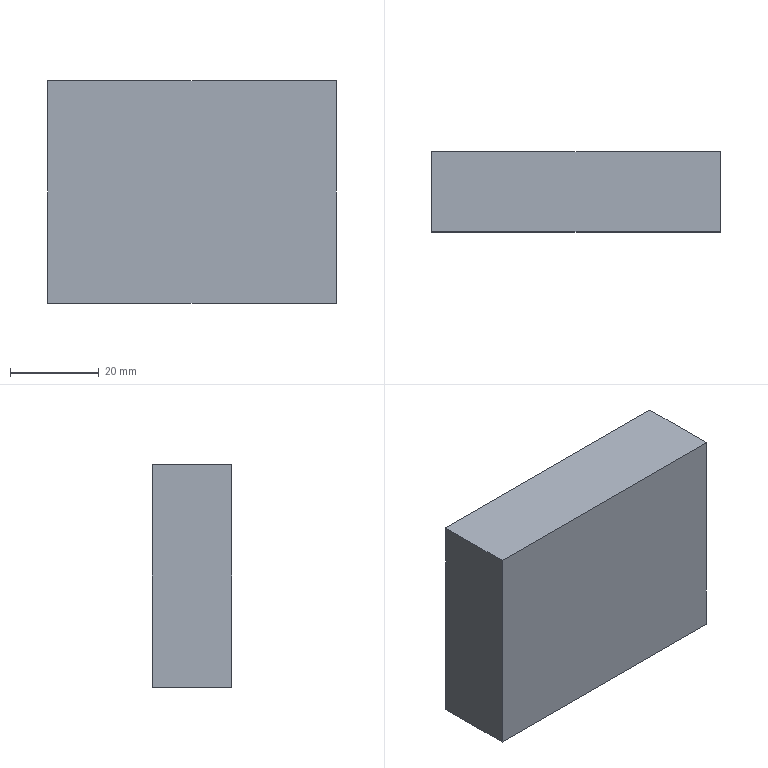Part | STEP file | Superstructure_3_1 | 1 solid | 6 faces | box 65 x 18 x 50 mm | volume 58500 mm3 | plane 6
STEP:
#1=CARTESIAN_POINT('',(0.,0.,0.));
#2=DIRECTION('',(0.,0.,1.));
#3=DIRECTION('',(1.,0.,0.));
#4=AXIS2_PLACEMENT_3D('',#1,#2,#3);
#5=CARTESIAN_POINT('',(-32.5,9.,50.));
#6=VERTEX_POINT('',#5);
#7=CARTESIAN_POINT('',(-32.5,-9.,50.));
#8=VERTEX_POINT('',#7);
#9=CARTESIAN_POINT('',(-32.5,9.,50.));
#10=DIRECTION('',(0.,-1.,0.));
#11=VECTOR('',#10,1.);
#12=LINE('',#9,#11);
#13=CARTESIAN_POINT('',(-32.5,9.,50.));
#14=DIRECTION('',(1.,0.,0.));
#15=DIRECTION('',(0.,0.,-1.));
#16=AXIS2_PLACEMENT_3D('',#13,#14,#15);
#17=PLANE('',#16);
#18=CARTESIAN_POINT('',(0.,0.));
#19=DIRECTION('',(0.,-1.));
#20=VECTOR('',#19,1.);
#21=LINE('',#18,#20);
#22=(GEOMETRIC_REPRESENTATION_CONTEXT(2)PARAMETRIC_REPRESENTATION_CONTEXT()REPRESENTATION_CONTEXT('',''));
#23=DEFINITIONAL_REPRESENTATION('',(#21),#22);
#24=PCURVE('',#17,#23);
#25=CARTESIAN_POINT('',(32.5,9.,50.));
#26=DIRECTION('',(0.,0.,-1.));
#27=DIRECTION('',(-1.,0.,0.));
#28=AXIS2_PLACEMENT_3D('',#25,#26,#27);
#29=PLANE('',#28);
#30=CARTESIAN_POINT('',(65.,0.));
#31=DIRECTION('',(0.,-1.));
#32=VECTOR('',#31,1.);
#33=LINE('',#30,#32);
#34=(GEOMETRIC_REPRESENTATION_CONTEXT(2)PARAMETRIC_REPRESENTATION_CONTEXT()REPRESENTATION_CONTEXT('',''));
#35=DEFINITIONAL_REPRESENTATION('',(#33),#34);
#36=PCURVE('',#29,#35);
#37=SURFACE_CURVE('',#12,(#24,#36),.PCURVE_S1.);
#38=EDGE_CURVE('',#6,#8,#37,.T.);
#39=ORIENTED_EDGE('',*,*,#38,.T.);
#40=CARTESIAN_POINT('',(-32.5,-9.,0.));
#41=VERTEX_POINT('',#40);
#42=CARTESIAN_POINT('',(-32.5,-9.,50.));
#43=DIRECTION('',(0.,0.,-1.));
#44=VECTOR('',#43,1.);
#45=LINE('',#42,#44);
#46=CARTESIAN_POINT('',(0.,-18.));
#47=DIRECTION('',(1.,0.));
#48=VECTOR('',#47,1.);
#49=LINE('',#46,#48);
#50=(GEOMETRIC_REPRESENTATION_CONTEXT(2)PARAMETRIC_REPRESENTATION_CONTEXT()REPRESENTATION_CONTEXT('',''));
#51=DEFINITIONAL_REPRESENTATION('',(#49),#50);
#52=PCURVE('',#17,#51);
#53=CARTESIAN_POINT('',(0.,-9.,25.));
#54=DIRECTION('',(0.,1.,0.));
#55=DIRECTION('',(0.,0.,1.));
#56=AXIS2_PLACEMENT_3D('',#53,#54,#55);
#57=PLANE('',#56);
#58=CARTESIAN_POINT('',(25.,-32.5));
#59=DIRECTION('',(-1.,0.));
#60=VECTOR('',#59,1.);
#61=LINE('',#58,#60);
#62=(GEOMETRIC_REPRESENTATION_CONTEXT(2)PARAMETRIC_REPRESENTATION_CONTEXT()REPRESENTATION_CONTEXT('',''));
#63=DEFINITIONAL_REPRESENTATION('',(#61),#62);
#64=PCURVE('',#57,#63);
#65=SURFACE_CURVE('',#45,(#52,#64),.PCURVE_S1.);
#66=EDGE_CURVE('',#8,#41,#65,.T.);
#67=ORIENTED_EDGE('',*,*,#66,.T.);
#68=CARTESIAN_POINT('',(-32.5,9.,0.));
#69=VERTEX_POINT('',#68);
#70=CARTESIAN_POINT('',(-32.5,9.,0.));
#71=DIRECTION('',(0.,-1.,0.));
#72=VECTOR('',#71,1.);
#73=LINE('',#70,#72);
#74=CARTESIAN_POINT('',(50.,0.));
#75=DIRECTION('',(0.,-1.));
#76=VECTOR('',#75,1.);
#77=LINE('',#74,#76);
#78=(GEOMETRIC_REPRESENTATION_CONTEXT(2)PARAMETRIC_REPRESENTATION_CONTEXT()REPRESENTATION_CONTEXT('',''));
#79=DEFINITIONAL_REPRESENTATION('',(#77),#78);
#80=PCURVE('',#17,#79);
#81=CARTESIAN_POINT('',(-32.5,9.,0.));
#82=DIRECTION('',(0.,0.,1.));
#83=DIRECTION('',(1.,0.,0.));
#84=AXIS2_PLACEMENT_3D('',#81,#82,#83);
#85=PLANE('',#84);
#86=CARTESIAN_POINT('',(0.,0.));
#87=DIRECTION('',(0.,-1.));
#88=VECTOR('',#87,1.);
#89=LINE('',#86,#88);
#90=(GEOMETRIC_REPRESENTATION_CONTEXT(2)PARAMETRIC_REPRESENTATION_CONTEXT()REPRESENTATION_CONTEXT('',''));
#91=DEFINITIONAL_REPRESENTATION('',(#89),#90);
#92=PCURVE('',#85,#91);
#93=SURFACE_CURVE('',#73,(#80,#92),.PCURVE_S1.);
#94=EDGE_CURVE('',#69,#41,#93,.T.);
#95=ORIENTED_EDGE('',*,*,#94,.F.);
#96=CARTESIAN_POINT('',(-32.5,9.,50.));
#97=DIRECTION('',(0.,0.,-1.));
#98=VECTOR('',#97,1.);
#99=LINE('',#96,#98);
#100=CARTESIAN_POINT('',(0.,0.));
#101=DIRECTION('',(1.,0.));
#102=VECTOR('',#101,1.);
#103=LINE('',#100,#102);
#104=(GEOMETRIC_REPRESENTATION_CONTEXT(2)PARAMETRIC_REPRESENTATION_CONTEXT()REPRESENTATION_CONTEXT('',''));
#105=DEFINITIONAL_REPRESENTATION('',(#103),#104);
#106=PCURVE('',#17,#105);
#107=CARTESIAN_POINT('',(0.,9.,25.));
#108=DIRECTION('',(0.,1.,0.));
#109=DIRECTION('',(0.,0.,1.));
#110=AXIS2_PLACEMENT_3D('',#107,#108,#109);
#111=PLANE('',#110);
#112=CARTESIAN_POINT('',(25.,-32.5));
#113=DIRECTION('',(-1.,0.));
#114=VECTOR('',#113,1.);
#115=LINE('',#112,#114);
#116=(GEOMETRIC_REPRESENTATION_CONTEXT(2)PARAMETRIC_REPRESENTATION_CONTEXT()REPRESENTATION_CONTEXT('',''));
#117=DEFINITIONAL_REPRESENTATION('',(#115),#116);
#118=PCURVE('',#111,#117);
#119=SURFACE_CURVE('',#99,(#106,#118),.PCURVE_S1.);
#120=EDGE_CURVE('',#6,#69,#119,.T.);
#121=ORIENTED_EDGE('',*,*,#120,.F.);
#122=EDGE_LOOP('',(#39,#67,#95,#121));
#123=FACE_BOUND('',#122,.F.);
#124=ADVANCED_FACE('',(#123),#17,.F.);
#125=ORIENTED_EDGE('',*,*,#94,.T.);
#126=CARTESIAN_POINT('',(32.5,-9.,0.));
#127=VERTEX_POINT('',#126);
#128=CARTESIAN_POINT('',(-32.5,-9.,0.));
#129=DIRECTION('',(1.,0.,0.));
#130=VECTOR('',#129,1.);
#131=LINE('',#128,#130);
#132=CARTESIAN_POINT('',(0.,-18.));
#133=DIRECTION('',(1.,0.));
#134=VECTOR('',#133,1.);
#135=LINE('',#132,#134);
#136=(GEOMETRIC_REPRESENTATION_CONTEXT(2)PARAMETRIC_REPRESENTATION_CONTEXT()REPRESENTATION_CONTEXT('',''));
#137=DEFINITIONAL_REPRESENTATION('',(#135),#136);
#138=PCURVE('',#85,#137);
#139=CARTESIAN_POINT('',(-25.,-32.5));
#140=DIRECTION('',(0.,1.));
#141=VECTOR('',#140,1.);
#142=LINE('',#139,#141);
#143=(GEOMETRIC_REPRESENTATION_CONTEXT(2)PARAMETRIC_REPRESENTATION_CONTEXT()REPRESENTATION_CONTEXT('',''));
#144=DEFINITIONAL_REPRESENTATION('',(#142),#143);
#145=PCURVE('',#57,#144);
#146=SURFACE_CURVE('',#131,(#138,#145),.PCURVE_S1.);
#147=EDGE_CURVE('',#41,#127,#146,.T.);
#148=ORIENTED_EDGE('',*,*,#147,.T.);
#149=CARTESIAN_POINT('',(32.5,9.,0.));
#150=VERTEX_POINT('',#149);
#151=CARTESIAN_POINT('',(32.5,9.,0.));
#152=DIRECTION('',(0.,-1.,0.));
#153=VECTOR('',#152,1.);
#154=LINE('',#151,#153);
#155=CARTESIAN_POINT('',(65.,0.));
#156=DIRECTION('',(0.,-1.));
#157=VECTOR('',#156,1.);
#158=LINE('',#155,#157);
#159=(GEOMETRIC_REPRESENTATION_CONTEXT(2)PARAMETRIC_REPRESENTATION_CONTEXT()REPRESENTATION_CONTEXT('',''));
#160=DEFINITIONAL_REPRESENTATION('',(#158),#159);
#161=PCURVE('',#85,#160);
#162=CARTESIAN_POINT('',(32.5,9.,0.));
#163=DIRECTION('',(-1.,0.,0.));
#164=DIRECTION('',(0.,0.,1.));
#165=AXIS2_PLACEMENT_3D('',#162,#163,#164);
#166=PLANE('',#165);
#167=CARTESIAN_POINT('',(0.,0.));
#168=DIRECTION('',(0.,-1.));
#169=VECTOR('',#168,1.);
#170=LINE('',#167,#169);
#171=(GEOMETRIC_REPRESENTATION_CONTEXT(2)PARAMETRIC_REPRESENTATION_CONTEXT()REPRESENTATION_CONTEXT('',''));
#172=DEFINITIONAL_REPRESENTATION('',(#170),#171);
#173=PCURVE('',#166,#172);
#174=SURFACE_CURVE('',#154,(#161,#173),.PCURVE_S1.);
#175=EDGE_CURVE('',#150,#127,#174,.T.);
#176=ORIENTED_EDGE('',*,*,#175,.F.);
#177=CARTESIAN_POINT('',(-32.5,9.,0.));
#178=DIRECTION('',(1.,0.,0.));
#179=VECTOR('',#178,1.);
#180=LINE('',#177,#179);
#181=CARTESIAN_POINT('',(0.,0.));
#182=DIRECTION('',(1.,0.));
#183=VECTOR('',#182,1.);
#184=LINE('',#181,#183);
#185=(GEOMETRIC_REPRESENTATION_CONTEXT(2)PARAMETRIC_REPRESENTATION_CONTEXT()REPRESENTATION_CONTEXT('',''));
#186=DEFINITIONAL_REPRESENTATION('',(#184),#185);
#187=PCURVE('',#85,#186);
#188=CARTESIAN_POINT('',(-25.,-32.5));
#189=DIRECTION('',(0.,1.));
#190=VECTOR('',#189,1.);
#191=LINE('',#188,#190);
#192=(GEOMETRIC_REPRESENTATION_CONTEXT(2)PARAMETRIC_REPRESENTATION_CONTEXT()REPRESENTATION_CONTEXT('',''));
#193=DEFINITIONAL_REPRESENTATION('',(#191),#192);
#194=PCURVE('',#111,#193);
#195=SURFACE_CURVE('',#180,(#187,#194),.PCURVE_S1.);
#196=EDGE_CURVE('',#69,#150,#195,.T.);
#197=ORIENTED_EDGE('',*,*,#196,.F.);
#198=EDGE_LOOP('',(#125,#148,#176,#197));
#199=FACE_BOUND('',#198,.F.);
#200=ADVANCED_FACE('',(#199),#85,.F.);
#201=ORIENTED_EDGE('',*,*,#175,.T.);
#202=CARTESIAN_POINT('',(32.5,-9.,50.));
#203=VERTEX_POINT('',#202);
#204=CARTESIAN_POINT('',(32.5,-9.,0.));
#205=DIRECTION('',(0.,0.,1.));
#206=VECTOR('',#205,1.);
#207=LINE('',#204,#206);
#208=CARTESIAN_POINT('',(0.,-18.));
#209=DIRECTION('',(1.,0.));
#210=VECTOR('',#209,1.);
#211=LINE('',#208,#210);
#212=(GEOMETRIC_REPRESENTATION_CONTEXT(2)PARAMETRIC_REPRESENTATION_CONTEXT()REPRESENTATION_CONTEXT('',''));
#213=DEFINITIONAL_REPRESENTATION('',(#211),#212);
#214=PCURVE('',#166,#213);
#215=CARTESIAN_POINT('',(-25.,32.5));
#216=DIRECTION('',(1.,0.));
#217=VECTOR('',#216,1.);
#218=LINE('',#215,#217);
#219=(GEOMETRIC_REPRESENTATION_CONTEXT(2)PARAMETRIC_REPRESENTATION_CONTEXT()REPRESENTATION_CONTEXT('',''));
#220=DEFINITIONAL_REPRESENTATION('',(#218),#219);
#221=PCURVE('',#57,#220);
#222=SURFACE_CURVE('',#207,(#214,#221),.PCURVE_S1.);
#223=EDGE_CURVE('',#127,#203,#222,.T.);
#224=ORIENTED_EDGE('',*,*,#223,.T.);
#225=CARTESIAN_POINT('',(32.5,9.,50.));
#226=VERTEX_POINT('',#225);
#227=CARTESIAN_POINT('',(32.5,9.,50.));
#228=DIRECTION('',(0.,-1.,0.));
#229=VECTOR('',#228,1.);
#230=LINE('',#227,#229);
#231=CARTESIAN_POINT('',(50.,0.));
#232=DIRECTION('',(0.,-1.));
#233=VECTOR('',#232,1.);
#234=LINE('',#231,#233);
#235=(GEOMETRIC_REPRESENTATION_CONTEXT(2)PARAMETRIC_REPRESENTATION_CONTEXT()REPRESENTATION_CONTEXT('',''));
#236=DEFINITIONAL_REPRESENTATION('',(#234),#235);
#237=PCURVE('',#166,#236);
#238=CARTESIAN_POINT('',(0.,0.));
#239=DIRECTION('',(0.,-1.));
#240=VECTOR('',#239,1.);
#241=LINE('',#238,#240);
#242=(GEOMETRIC_REPRESENTATION_CONTEXT(2)PARAMETRIC_REPRESENTATION_CONTEXT()REPRESENTATION_CONTEXT('',''));
#243=DEFINITIONAL_REPRESENTATION('',(#241),#242);
#244=PCURVE('',#29,#243);
#245=SURFACE_CURVE('',#230,(#237,#244),.PCURVE_S1.);
#246=EDGE_CURVE('',#226,#203,#245,.T.);
#247=ORIENTED_EDGE('',*,*,#246,.F.);
#248=CARTESIAN_POINT('',(32.5,9.,0.));
#249=DIRECTION('',(0.,0.,1.));
#250=VECTOR('',#249,1.);
#251=LINE('',#248,#250);
#252=CARTESIAN_POINT('',(0.,0.));
#253=DIRECTION('',(1.,0.));
#254=VECTOR('',#253,1.);
#255=LINE('',#252,#254);
#256=(GEOMETRIC_REPRESENTATION_CONTEXT(2)PARAMETRIC_REPRESENTATION_CONTEXT()REPRESENTATION_CONTEXT('',''));
#257=DEFINITIONAL_REPRESENTATION('',(#255),#256);
#258=PCURVE('',#166,#257);
#259=CARTESIAN_POINT('',(-25.,32.5));
#260=DIRECTION('',(1.,0.));
#261=VECTOR('',#260,1.);
#262=LINE('',#259,#261);
#263=(GEOMETRIC_REPRESENTATION_CONTEXT(2)PARAMETRIC_REPRESENTATION_CONTEXT()REPRESENTATION_CONTEXT('',''));
#264=DEFINITIONAL_REPRESENTATION('',(#262),#263);
#265=PCURVE('',#111,#264);
#266=SURFACE_CURVE('',#251,(#258,#265),.PCURVE_S1.);
#267=EDGE_CURVE('',#150,#226,#266,.T.);
#268=ORIENTED_EDGE('',*,*,#267,.F.);
#269=EDGE_LOOP('',(#201,#224,#247,#268));
#270=FACE_BOUND('',#269,.F.);
#271=ADVANCED_FACE('',(#270),#166,.F.);
#272=ORIENTED_EDGE('',*,*,#246,.T.);
#273=CARTESIAN_POINT('',(32.5,-9.,50.));
#274=DIRECTION('',(-1.,0.,0.));
#275=VECTOR('',#274,1.);
#276=LINE('',#273,#275);
#277=CARTESIAN_POINT('',(0.,-18.));
#278=DIRECTION('',(1.,0.));
#279=VECTOR('',#278,1.);
#280=LINE('',#277,#279);
#281=(GEOMETRIC_REPRESENTATION_CONTEXT(2)PARAMETRIC_REPRESENTATION_CONTEXT()REPRESENTATION_CONTEXT('',''));
#282=DEFINITIONAL_REPRESENTATION('',(#280),#281);
#283=PCURVE('',#29,#282);
#284=CARTESIAN_POINT('',(25.,32.5));
#285=DIRECTION('',(0.,-1.));
#286=VECTOR('',#285,1.);
#287=LINE('',#284,#286);
#288=(GEOMETRIC_REPRESENTATION_CONTEXT(2)PARAMETRIC_REPRESENTATION_CONTEXT()REPRESENTATION_CONTEXT('',''));
#289=DEFINITIONAL_REPRESENTATION('',(#287),#288);
#290=PCURVE('',#57,#289);
#291=SURFACE_CURVE('',#276,(#283,#290),.PCURVE_S1.);
#292=EDGE_CURVE('',#203,#8,#291,.T.);
#293=ORIENTED_EDGE('',*,*,#292,.T.);
#294=ORIENTED_EDGE('',*,*,#38,.F.);
#295=CARTESIAN_POINT('',(32.5,9.,50.));
#296=DIRECTION('',(-1.,0.,0.));
#297=VECTOR('',#296,1.);
#298=LINE('',#295,#297);
#299=CARTESIAN_POINT('',(0.,0.));
#300=DIRECTION('',(1.,0.));
#301=VECTOR('',#300,1.);
#302=LINE('',#299,#301);
#303=(GEOMETRIC_REPRESENTATION_CONTEXT(2)PARAMETRIC_REPRESENTATION_CONTEXT()REPRESENTATION_CONTEXT('',''));
#304=DEFINITIONAL_REPRESENTATION('',(#302),#303);
#305=PCURVE('',#29,#304);
#306=CARTESIAN_POINT('',(25.,32.5));
#307=DIRECTION('',(0.,-1.));
#308=VECTOR('',#307,1.);
#309=LINE('',#306,#308);
#310=(GEOMETRIC_REPRESENTATION_CONTEXT(2)PARAMETRIC_REPRESENTATION_CONTEXT()REPRESENTATION_CONTEXT('',''));
#311=DEFINITIONAL_REPRESENTATION('',(#309),#310);
#312=PCURVE('',#111,#311);
#313=SURFACE_CURVE('',#298,(#305,#312),.PCURVE_S1.);
#314=EDGE_CURVE('',#226,#6,#313,.T.);
#315=ORIENTED_EDGE('',*,*,#314,.F.);
#316=EDGE_LOOP('',(#272,#293,#294,#315));
#317=FACE_BOUND('',#316,.F.);
#318=ADVANCED_FACE('',(#317),#29,.F.);
#319=ORIENTED_EDGE('',*,*,#120,.T.);
#320=ORIENTED_EDGE('',*,*,#196,.T.);
#321=ORIENTED_EDGE('',*,*,#267,.T.);
#322=ORIENTED_EDGE('',*,*,#314,.T.);
#323=EDGE_LOOP('',(#319,#320,#321,#322));
#324=FACE_BOUND('',#323,.F.);
#325=ADVANCED_FACE('',(#324),#111,.T.);
#326=ORIENTED_EDGE('',*,*,#66,.T.);
#327=ORIENTED_EDGE('',*,*,#147,.T.);
#328=ORIENTED_EDGE('',*,*,#223,.T.);
#329=ORIENTED_EDGE('',*,*,#292,.T.);
#330=EDGE_LOOP('',(#326,#327,#328,#329));
#331=FACE_BOUND('',#330,.T.);
#332=ADVANCED_FACE('',(#331),#57,.F.);
#333=CLOSED_SHELL('',(#124,#200,#271,#318,#325,#332));
#334=MANIFOLD_SOLID_BREP('',#333);
#335=(LENGTH_UNIT()NAMED_UNIT(*)SI_UNIT(.MILLI.,.METRE.));
#336=UNCERTAINTY_MEASURE_WITH_UNIT(LENGTH_MEASURE(0.0000001),#335,'','');
#337=(NAMED_UNIT(*)PLANE_ANGLE_UNIT()SI_UNIT($,.RADIAN.));
#338=(NAMED_UNIT(*)SI_UNIT($,.STERADIAN.)SOLID_ANGLE_UNIT());
#339=(GEOMETRIC_REPRESENTATION_CONTEXT(3)GLOBAL_UNCERTAINTY_ASSIGNED_CONTEXT((#336))GLOBAL_UNIT_ASSIGNED_CONTEXT((#335,#337,#338))REPRESENTATION_CONTEXT('',''));
#340=ADVANCED_BREP_SHAPE_REPRESENTATION('',(#4,#334),#339);